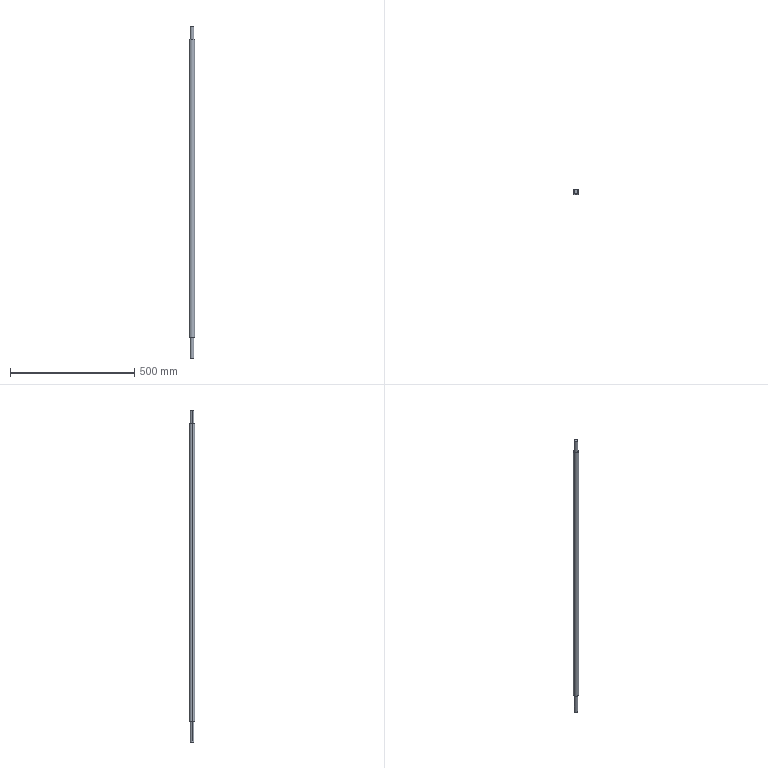Part | SolidWorks | features BaseBody 1, ICE 1, MoveFace 1 | 1 solid | 14 faces | box 22.084 x 22.084 x 1336 mm | volume 483171 mm3 | plane 8 | cylinder 6 | commonest cylinder face diameters 15 x4 22.084 x2
STEP:
#1=CARTESIAN_POINT('',(-187.358,334.799,-600.));
#2=VERTEX_POINT('',#1);
#3=CARTESIAN_POINT('',(-209.442,334.799,-600.));
#4=VERTEX_POINT('',#3);
#5=CARTESIAN_POINT('',(-198.4,334.799,-600.));
#6=DIRECTION('',(0.,0.,1.));
#7=DIRECTION('',(1.,0.,0.));
#8=AXIS2_PLACEMENT_3D('',#5,#6,#7);
#9=CIRCLE('',#8,11.042);
#10=EDGE_CURVE('',#2,#4,#9,.T.);
#11=ORIENTED_EDGE('',*,*,#10,.T.);
#12=CARTESIAN_POINT('',(-209.442,334.799,600.));
#13=VERTEX_POINT('',#12);
#14=CARTESIAN_POINT('',(-209.442,334.799,0.));
#15=DIRECTION('',(0.,0.,1.));
#16=VECTOR('',#15,1000.);
#17=LINE('',#14,#16);
#18=EDGE_CURVE('',#4,#13,#17,.T.);
#19=ORIENTED_EDGE('',*,*,#18,.T.);
#20=CARTESIAN_POINT('',(-187.358,334.799,600.));
#21=VERTEX_POINT('',#20);
#22=CARTESIAN_POINT('',(-198.4,334.799,600.));
#23=DIRECTION('',(0.,0.,-1.));
#24=DIRECTION('',(1.,0.,0.));
#25=AXIS2_PLACEMENT_3D('',#22,#23,#24);
#26=CIRCLE('',#25,11.042);
#27=EDGE_CURVE('',#13,#21,#26,.T.);
#28=ORIENTED_EDGE('',*,*,#27,.T.);
#29=CARTESIAN_POINT('',(-187.358,334.799,0.));
#30=DIRECTION('',(0.,0.,1.));
#31=VECTOR('',#30,1000.);
#32=LINE('',#29,#31);
#33=EDGE_CURVE('',#2,#21,#32,.T.);
#34=ORIENTED_EDGE('',*,*,#33,.F.);
#35=EDGE_LOOP('',(#11,#19,#28,#34));
#36=FACE_OUTER_BOUND('',#35,.T.);
#37=CARTESIAN_POINT('',(-198.4,334.799,0.));
#38=DIRECTION('',(0.,0.,1.));
#39=DIRECTION('',(1.,0.,0.));
#40=AXIS2_PLACEMENT_3D('',#37,#38,#39);
#41=CYLINDRICAL_SURFACE('',#40,11.042);
#42=ADVANCED_FACE('',(#36),#41,.T.);
#43=CARTESIAN_POINT('',(-205.9,334.799,-600.));
#44=VERTEX_POINT('',#43);
#45=CARTESIAN_POINT('',(-190.9,334.799,-600.));
#46=VERTEX_POINT('',#45);
#47=CARTESIAN_POINT('',(-198.4,334.799,-600.));
#48=DIRECTION('',(0.,0.,-1.));
#49=DIRECTION('',(-1.,0.,0.));
#50=AXIS2_PLACEMENT_3D('',#47,#48,#49);
#51=CIRCLE('',#50,7.5);
#52=EDGE_CURVE('',#44,#46,#51,.T.);
#53=ORIENTED_EDGE('',*,*,#52,.T.);
#54=CARTESIAN_POINT('',(-190.9,334.799,-683.1));
#55=VERTEX_POINT('',#54);
#56=CARTESIAN_POINT('',(-190.9,334.799,-600.));
#57=DIRECTION('',(0.,0.,-1.));
#58=VECTOR('',#57,1000.);
#59=LINE('',#56,#58);
#60=EDGE_CURVE('',#46,#55,#59,.T.);
#61=ORIENTED_EDGE('',*,*,#60,.T.);
#62=CARTESIAN_POINT('',(-195.9,341.87,-683.1));
#63=VERTEX_POINT('',#62);
#64=CARTESIAN_POINT('',(-198.4,334.799,-683.1));
#65=DIRECTION('',(0.,0.,1.));
#66=DIRECTION('',(-1.,0.,0.));
#67=AXIS2_PLACEMENT_3D('',#64,#65,#66);
#68=CIRCLE('',#67,7.5);
#69=EDGE_CURVE('',#55,#63,#68,.T.);
#70=ORIENTED_EDGE('',*,*,#69,.T.);
#71=CARTESIAN_POINT('',(-195.9,341.87,-648.1));
#72=VERTEX_POINT('',#71);
#73=CARTESIAN_POINT('',(-195.9,341.87,-600.));
#74=DIRECTION('',(0.,0.,-1.));
#75=VECTOR('',#74,1000.);
#76=LINE('',#73,#75);
#77=EDGE_CURVE('',#72,#63,#76,.T.);
#78=ORIENTED_EDGE('',*,*,#77,.F.);
#79=CARTESIAN_POINT('',(-200.9,341.87,-648.1));
#80=VERTEX_POINT('',#79);
#81=CARTESIAN_POINT('',(-198.4,334.799,-648.1));
#82=DIRECTION('',(0.,0.,1.));
#83=DIRECTION('',(-1.,0.,0.));
#84=AXIS2_PLACEMENT_3D('',#81,#82,#83);
#85=CIRCLE('',#84,7.5);
#86=EDGE_CURVE('',#72,#80,#85,.T.);
#87=ORIENTED_EDGE('',*,*,#86,.T.);
#88=CARTESIAN_POINT('',(-200.9,341.87,-683.1));
#89=VERTEX_POINT('',#88);
#90=CARTESIAN_POINT('',(-200.9,341.87,-600.));
#91=DIRECTION('',(0.,0.,1.));
#92=VECTOR('',#91,1000.);
#93=LINE('',#90,#92);
#94=EDGE_CURVE('',#89,#80,#93,.T.);
#95=ORIENTED_EDGE('',*,*,#94,.F.);
#96=CARTESIAN_POINT('',(-205.9,334.799,-683.1));
#97=VERTEX_POINT('',#96);
#98=CARTESIAN_POINT('',(-198.4,334.799,-683.1));
#99=DIRECTION('',(0.,0.,1.));
#100=DIRECTION('',(-1.,0.,0.));
#101=AXIS2_PLACEMENT_3D('',#98,#99,#100);
#102=CIRCLE('',#101,7.5);
#103=EDGE_CURVE('',#89,#97,#102,.T.);
#104=ORIENTED_EDGE('',*,*,#103,.T.);
#105=CARTESIAN_POINT('',(-205.9,334.799,-600.));
#106=DIRECTION('',(0.,0.,-1.));
#107=VECTOR('',#106,1000.);
#108=LINE('',#105,#107);
#109=EDGE_CURVE('',#44,#97,#108,.T.);
#110=ORIENTED_EDGE('',*,*,#109,.F.);
#111=EDGE_LOOP('',(#53,#61,#70,#78,#87,#95,#104,#110));
#112=FACE_OUTER_BOUND('',#111,.T.);
#113=CARTESIAN_POINT('',(-198.4,334.799,-600.));
#114=DIRECTION('',(0.,0.,-1.));
#115=DIRECTION('',(-1.,0.,0.));
#116=AXIS2_PLACEMENT_3D('',#113,#114,#115);
#117=CYLINDRICAL_SURFACE('',#116,7.5);
#118=ADVANCED_FACE('',(#112),#117,.T.);
#119=CARTESIAN_POINT('',(-205.9,334.799,600.));
#120=VERTEX_POINT('',#119);
#121=CARTESIAN_POINT('',(-190.9,334.799,600.));
#122=VERTEX_POINT('',#121);
#123=CARTESIAN_POINT('',(-198.4,334.799,600.));
#124=DIRECTION('',(0.,0.,-1.));
#125=DIRECTION('',(1.,0.,0.));
#126=AXIS2_PLACEMENT_3D('',#123,#124,#125);
#127=CIRCLE('',#126,7.5);
#128=EDGE_CURVE('',#120,#122,#127,.T.);
#129=ORIENTED_EDGE('',*,*,#128,.F.);
#130=CARTESIAN_POINT('',(-205.9,334.799,652.863));
#131=VERTEX_POINT('',#130);
#132=CARTESIAN_POINT('',(-205.9,334.799,600.));
#133=DIRECTION('',(0.,0.,1.));
#134=VECTOR('',#133,1000.);
#135=LINE('',#132,#134);
#136=EDGE_CURVE('',#120,#131,#135,.T.);
#137=ORIENTED_EDGE('',*,*,#136,.T.);
#138=CARTESIAN_POINT('',(-190.9,334.799,652.863));
#139=VERTEX_POINT('',#138);
#140=CARTESIAN_POINT('',(-198.4,334.799,652.863));
#141=DIRECTION('',(0.,0.,-1.));
#142=DIRECTION('',(1.,0.,0.));
#143=AXIS2_PLACEMENT_3D('',#140,#141,#142);
#144=CIRCLE('',#143,7.5);
#145=EDGE_CURVE('',#131,#139,#144,.T.);
#146=ORIENTED_EDGE('',*,*,#145,.T.);
#147=CARTESIAN_POINT('',(-190.9,334.799,600.));
#148=DIRECTION('',(0.,0.,1.));
#149=VECTOR('',#148,1000.);
#150=LINE('',#147,#149);
#151=EDGE_CURVE('',#122,#139,#150,.T.);
#152=ORIENTED_EDGE('',*,*,#151,.F.);
#153=EDGE_LOOP('',(#129,#137,#146,#152));
#154=FACE_OUTER_BOUND('',#153,.T.);
#155=CARTESIAN_POINT('',(-198.4,334.799,600.));
#156=DIRECTION('',(0.,0.,1.));
#157=DIRECTION('',(1.,0.,0.));
#158=AXIS2_PLACEMENT_3D('',#155,#156,#157);
#159=CYLINDRICAL_SURFACE('',#158,7.5);
#160=ADVANCED_FACE('',(#154),#159,.T.);
#161=ORIENTED_EDGE('',*,*,#18,.F.);
#162=CARTESIAN_POINT('',(-198.4,334.799,-600.));
#163=DIRECTION('',(0.,0.,1.));
#164=DIRECTION('',(1.,0.,0.));
#165=AXIS2_PLACEMENT_3D('',#162,#163,#164);
#166=CIRCLE('',#165,11.042);
#167=EDGE_CURVE('',#4,#2,#166,.T.);
#168=ORIENTED_EDGE('',*,*,#167,.T.);
#169=ORIENTED_EDGE('',*,*,#33,.T.);
#170=CARTESIAN_POINT('',(-198.4,334.799,600.));
#171=DIRECTION('',(0.,0.,-1.));
#172=DIRECTION('',(1.,0.,0.));
#173=AXIS2_PLACEMENT_3D('',#170,#171,#172);
#174=CIRCLE('',#173,11.042);
#175=EDGE_CURVE('',#21,#13,#174,.T.);
#176=ORIENTED_EDGE('',*,*,#175,.T.);
#177=EDGE_LOOP('',(#161,#168,#169,#176));
#178=FACE_OUTER_BOUND('',#177,.T.);
#179=CARTESIAN_POINT('',(-198.4,334.799,0.));
#180=DIRECTION('',(0.,0.,1.));
#181=DIRECTION('',(1.,0.,0.));
#182=AXIS2_PLACEMENT_3D('',#179,#180,#181);
#183=CYLINDRICAL_SURFACE('',#182,11.042);
#184=ADVANCED_FACE('',(#178),#183,.T.);
#185=ORIENTED_EDGE('',*,*,#52,.F.);
#186=CARTESIAN_POINT('',(-198.4,334.799,-600.));
#187=DIRECTION('',(0.,0.,-1.));
#188=DIRECTION('',(-1.,0.,0.));
#189=AXIS2_PLACEMENT_3D('',#186,#187,#188);
#190=CIRCLE('',#189,7.5);
#191=EDGE_CURVE('',#46,#44,#190,.T.);
#192=ORIENTED_EDGE('',*,*,#191,.F.);
#193=EDGE_LOOP('',(#185,#192));
#194=FACE_BOUND('',#193,.T.);
#195=ORIENTED_EDGE('',*,*,#10,.F.);
#196=ORIENTED_EDGE('',*,*,#167,.F.);
#197=EDGE_LOOP('',(#195,#196));
#198=FACE_OUTER_BOUND('',#197,.T.);
#199=CARTESIAN_POINT('',(-198.4,334.799,-600.));
#200=DIRECTION('',(0.,0.,1.));
#201=DIRECTION('',(1.,0.,0.));
#202=AXIS2_PLACEMENT_3D('',#199,#200,#201);
#203=PLANE('',#202);
#204=ADVANCED_FACE('',(#194,#198),#203,.F.);
#205=CARTESIAN_POINT('',(-198.4,334.799,600.));
#206=DIRECTION('',(0.,0.,-1.));
#207=DIRECTION('',(1.,0.,0.));
#208=AXIS2_PLACEMENT_3D('',#205,#206,#207);
#209=CIRCLE('',#208,7.5);
#210=EDGE_CURVE('',#122,#120,#209,.T.);
#211=ORIENTED_EDGE('',*,*,#210,.T.);
#212=ORIENTED_EDGE('',*,*,#128,.T.);
#213=EDGE_LOOP('',(#211,#212));
#214=FACE_BOUND('',#213,.T.);
#215=ORIENTED_EDGE('',*,*,#175,.F.);
#216=ORIENTED_EDGE('',*,*,#27,.F.);
#217=EDGE_LOOP('',(#215,#216));
#218=FACE_OUTER_BOUND('',#217,.T.);
#219=CARTESIAN_POINT('',(-198.4,334.799,600.));
#220=DIRECTION('',(0.,0.,1.));
#221=DIRECTION('',(1.,0.,0.));
#222=AXIS2_PLACEMENT_3D('',#219,#220,#221);
#223=PLANE('',#222);
#224=ADVANCED_FACE('',(#214,#218),#223,.T.);
#225=ORIENTED_EDGE('',*,*,#60,.F.);
#226=ORIENTED_EDGE('',*,*,#191,.T.);
#227=ORIENTED_EDGE('',*,*,#109,.T.);
#228=CARTESIAN_POINT('',(-198.4,334.799,-683.1));
#229=DIRECTION('',(0.,0.,1.));
#230=DIRECTION('',(-1.,0.,0.));
#231=AXIS2_PLACEMENT_3D('',#228,#229,#230);
#232=CIRCLE('',#231,7.5);
#233=EDGE_CURVE('',#97,#55,#232,.T.);
#234=ORIENTED_EDGE('',*,*,#233,.T.);
#235=EDGE_LOOP('',(#225,#226,#227,#234));
#236=FACE_OUTER_BOUND('',#235,.T.);
#237=CARTESIAN_POINT('',(-198.4,334.799,-600.));
#238=DIRECTION('',(0.,0.,-1.));
#239=DIRECTION('',(-1.,0.,0.));
#240=AXIS2_PLACEMENT_3D('',#237,#238,#239);
#241=CYLINDRICAL_SURFACE('',#240,7.5);
#242=ADVANCED_FACE('',(#236),#241,.T.);
#243=ORIENTED_EDGE('',*,*,#136,.F.);
#244=ORIENTED_EDGE('',*,*,#210,.F.);
#245=ORIENTED_EDGE('',*,*,#151,.T.);
#246=CARTESIAN_POINT('',(-198.4,334.799,652.863));
#247=DIRECTION('',(0.,0.,-1.));
#248=DIRECTION('',(1.,0.,0.));
#249=AXIS2_PLACEMENT_3D('',#246,#247,#248);
#250=CIRCLE('',#249,7.5);
#251=EDGE_CURVE('',#139,#131,#250,.T.);
#252=ORIENTED_EDGE('',*,*,#251,.T.);
#253=EDGE_LOOP('',(#243,#244,#245,#252));
#254=FACE_OUTER_BOUND('',#253,.T.);
#255=CARTESIAN_POINT('',(-198.4,334.799,600.));
#256=DIRECTION('',(0.,0.,1.));
#257=DIRECTION('',(1.,0.,0.));
#258=AXIS2_PLACEMENT_3D('',#255,#256,#257);
#259=CYLINDRICAL_SURFACE('',#258,7.5);
#260=ADVANCED_FACE('',(#254),#259,.T.);
#261=CARTESIAN_POINT('',(-195.9,339.299,-683.1));
#262=VERTEX_POINT('',#261);
#263=CARTESIAN_POINT('',(-195.9,342.299,-683.1));
#264=DIRECTION('',(0.,-1.,0.));
#265=VECTOR('',#264,1000.);
#266=LINE('',#263,#265);
#267=EDGE_CURVE('',#63,#262,#266,.T.);
#268=ORIENTED_EDGE('',*,*,#267,.F.);
#269=ORIENTED_EDGE('',*,*,#69,.F.);
#270=ORIENTED_EDGE('',*,*,#233,.F.);
#271=ORIENTED_EDGE('',*,*,#103,.F.);
#272=CARTESIAN_POINT('',(-200.9,339.299,-683.1));
#273=VERTEX_POINT('',#272);
#274=CARTESIAN_POINT('',(-200.9,342.299,-683.1));
#275=DIRECTION('',(0.,1.,0.));
#276=VECTOR('',#275,1000.);
#277=LINE('',#274,#276);
#278=EDGE_CURVE('',#273,#89,#277,.T.);
#279=ORIENTED_EDGE('',*,*,#278,.F.);
#280=CARTESIAN_POINT('',(-195.9,339.299,-683.1));
#281=DIRECTION('',(-1.,0.,0.));
#282=VECTOR('',#281,1000.);
#283=LINE('',#280,#282);
#284=EDGE_CURVE('',#262,#273,#283,.T.);
#285=ORIENTED_EDGE('',*,*,#284,.F.);
#286=EDGE_LOOP('',(#268,#269,#270,#271,#279,#285));
#287=FACE_OUTER_BOUND('',#286,.T.);
#288=CARTESIAN_POINT('',(-198.4,334.799,-683.1));
#289=DIRECTION('',(0.,0.,-1.));
#290=DIRECTION('',(-1.,0.,0.));
#291=AXIS2_PLACEMENT_3D('',#288,#289,#290);
#292=PLANE('',#291);
#293=ADVANCED_FACE('',(#287),#292,.T.);
#294=ORIENTED_EDGE('',*,*,#251,.F.);
#295=ORIENTED_EDGE('',*,*,#145,.F.);
#296=EDGE_LOOP('',(#294,#295));
#297=FACE_OUTER_BOUND('',#296,.T.);
#298=CARTESIAN_POINT('',(-198.4,334.799,652.863));
#299=DIRECTION('',(0.,0.,1.));
#300=DIRECTION('',(1.,0.,0.));
#301=AXIS2_PLACEMENT_3D('',#298,#299,#300);
#302=PLANE('',#301);
#303=ADVANCED_FACE('',(#297),#302,.T.);
#304=ORIENTED_EDGE('',*,*,#77,.T.);
#305=ORIENTED_EDGE('',*,*,#267,.T.);
#306=CARTESIAN_POINT('',(-195.9,339.299,-648.1));
#307=VERTEX_POINT('',#306);
#308=CARTESIAN_POINT('',(-195.9,339.299,-648.1));
#309=DIRECTION('',(0.,0.,-1.));
#310=VECTOR('',#309,1000.);
#311=LINE('',#308,#310);
#312=EDGE_CURVE('',#307,#262,#311,.T.);
#313=ORIENTED_EDGE('',*,*,#312,.F.);
#314=CARTESIAN_POINT('',(-195.9,342.299,-648.1));
#315=DIRECTION('',(0.,-1.,0.));
#316=VECTOR('',#315,1000.);
#317=LINE('',#314,#316);
#318=EDGE_CURVE('',#72,#307,#317,.T.);
#319=ORIENTED_EDGE('',*,*,#318,.F.);
#320=EDGE_LOOP('',(#304,#305,#313,#319));
#321=FACE_OUTER_BOUND('',#320,.T.);
#322=CARTESIAN_POINT('',(-195.9,342.299,-648.1));
#323=DIRECTION('',(1.,0.,0.));
#324=DIRECTION('',(0.,0.,-1.));
#325=AXIS2_PLACEMENT_3D('',#322,#323,#324);
#326=PLANE('',#325);
#327=ADVANCED_FACE('',(#321),#326,.F.);
#328=ORIENTED_EDGE('',*,*,#94,.T.);
#329=CARTESIAN_POINT('',(-200.9,339.299,-648.1));
#330=VERTEX_POINT('',#329);
#331=CARTESIAN_POINT('',(-200.9,342.299,-648.1));
#332=DIRECTION('',(0.,1.,0.));
#333=VECTOR('',#332,1000.);
#334=LINE('',#331,#333);
#335=EDGE_CURVE('',#330,#80,#334,.T.);
#336=ORIENTED_EDGE('',*,*,#335,.F.);
#337=CARTESIAN_POINT('',(-200.9,339.299,-648.1));
#338=DIRECTION('',(0.,0.,-1.));
#339=VECTOR('',#338,1000.);
#340=LINE('',#337,#339);
#341=EDGE_CURVE('',#330,#273,#340,.T.);
#342=ORIENTED_EDGE('',*,*,#341,.T.);
#343=ORIENTED_EDGE('',*,*,#278,.T.);
#344=EDGE_LOOP('',(#328,#336,#342,#343));
#345=FACE_OUTER_BOUND('',#344,.T.);
#346=CARTESIAN_POINT('',(-200.9,342.299,-648.1));
#347=DIRECTION('',(-1.,0.,0.));
#348=DIRECTION('',(0.,0.,1.));
#349=AXIS2_PLACEMENT_3D('',#346,#347,#348);
#350=PLANE('',#349);
#351=ADVANCED_FACE('',(#345),#350,.F.);
#352=ORIENTED_EDGE('',*,*,#284,.T.);
#353=ORIENTED_EDGE('',*,*,#341,.F.);
#354=CARTESIAN_POINT('',(-195.9,339.299,-648.1));
#355=DIRECTION('',(-1.,0.,0.));
#356=VECTOR('',#355,1000.);
#357=LINE('',#354,#356);
#358=EDGE_CURVE('',#307,#330,#357,.T.);
#359=ORIENTED_EDGE('',*,*,#358,.F.);
#360=ORIENTED_EDGE('',*,*,#312,.T.);
#361=EDGE_LOOP('',(#352,#353,#359,#360));
#362=FACE_OUTER_BOUND('',#361,.T.);
#363=CARTESIAN_POINT('',(-195.9,339.299,-648.1));
#364=DIRECTION('',(0.,-1.,0.));
#365=DIRECTION('',(0.,0.,-1.));
#366=AXIS2_PLACEMENT_3D('',#363,#364,#365);
#367=PLANE('',#366);
#368=ADVANCED_FACE('',(#362),#367,.F.);
#369=ORIENTED_EDGE('',*,*,#318,.T.);
#370=ORIENTED_EDGE('',*,*,#358,.T.);
#371=ORIENTED_EDGE('',*,*,#335,.T.);
#372=ORIENTED_EDGE('',*,*,#86,.F.);
#373=EDGE_LOOP('',(#369,#370,#371,#372));
#374=FACE_OUTER_BOUND('',#373,.T.);
#375=CARTESIAN_POINT('',(0.,0.,-648.1));
#376=DIRECTION('',(0.,0.,-1.));
#377=DIRECTION('',(-1.,0.,0.));
#378=AXIS2_PLACEMENT_3D('',#375,#376,#377);
#379=PLANE('',#378);
#380=ADVANCED_FACE('',(#374),#379,.T.);
#381=CLOSED_SHELL('',(#42,#118,#160,#184,#204,#224,#242,#260,#293,#303,#327,#351,#368,#380));
#382=MANIFOLD_SOLID_BREP('',#381);
#383=CARTESIAN_POINT('',(0.,0.,0.));
#384=DIRECTION('',(0.,0.,1.));
#385=DIRECTION('',(1.,0.,0.));
#386=AXIS2_PLACEMENT_3D('',#383,#384,#385);
#387=(LENGTH_UNIT()NAMED_UNIT(*)SI_UNIT(.MILLI.,.METRE.));
#388=UNCERTAINTY_MEASURE_WITH_UNIT(LENGTH_MEASURE(0.00001),#387,'','');
#389=(NAMED_UNIT(*)PLANE_ANGLE_UNIT()SI_UNIT($,.RADIAN.));
#390=(NAMED_UNIT(*)SI_UNIT($,.STERADIAN.)SOLID_ANGLE_UNIT());
#391=(GEOMETRIC_REPRESENTATION_CONTEXT(3)GLOBAL_UNCERTAINTY_ASSIGNED_CONTEXT((#388))GLOBAL_UNIT_ASSIGNED_CONTEXT((#387,#389,#390))REPRESENTATION_CONTEXT('',''));
#392=ADVANCED_BREP_SHAPE_REPRESENTATION('',(#382,#386),#391);